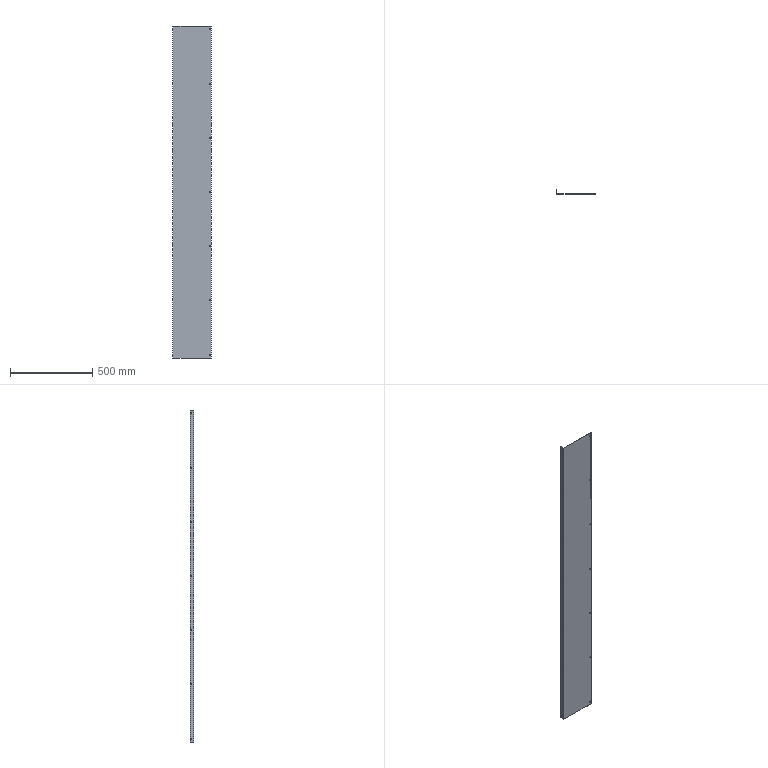Part | 1 solid | 70 faces | box 234 x 24 x 2016 mm | volume 516858 mm3 | plane 40 | cylinder 30 | commonest cylinder face diameters 6 x28 0.4 x1 2.4 x1